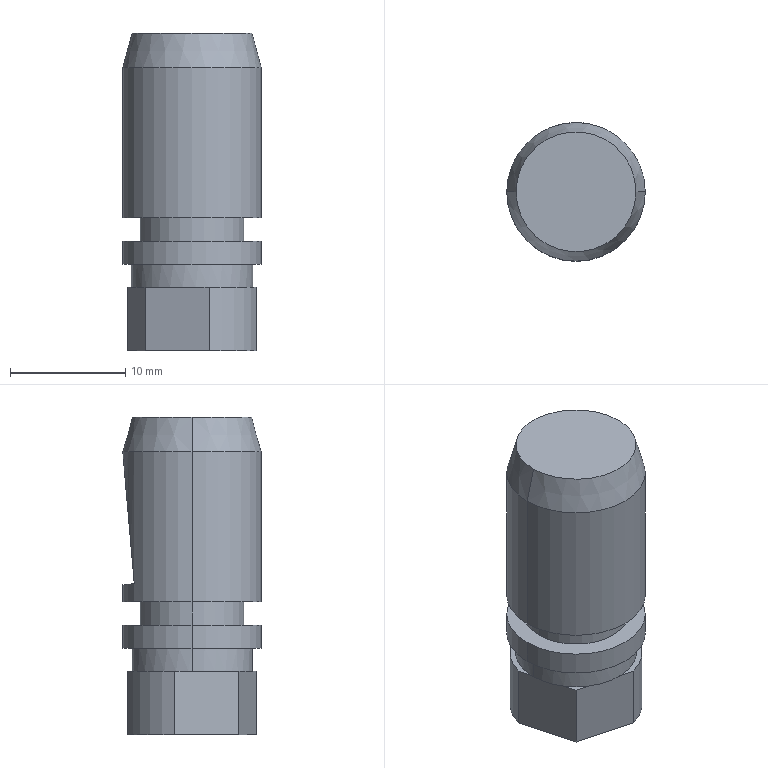Part | STEP file | OP10-114_dia-pin | 1 solid | 31 faces | box 12 x 12 x 27.5 mm | volume 2777 mm3 | plane 19 | cylinder 10 | cone 2 | commonest cylinder face diameters 12 x4 9 x2 10.5 x2 11.5 x2